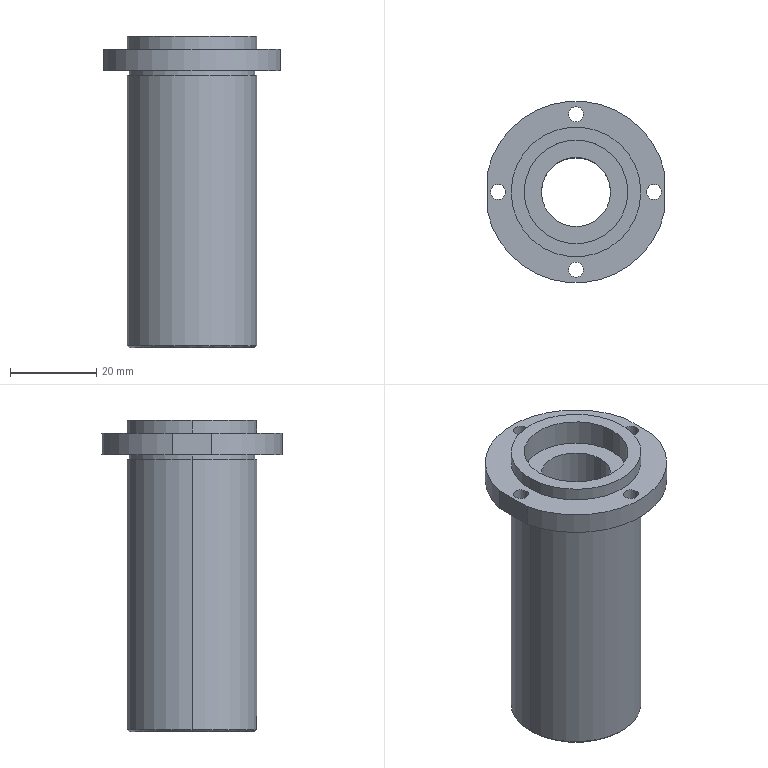Part | STEP file | 06-01-04 rotary shaft sleeve | 1 solid | 33 faces | box 41 x 42 x 72 mm | volume 36513 mm3 | cylinder 22 | plane 9 | cone 2 | commonest cylinder face diameters 3.5 x8 24 x4 30 x4 16 x2 29 x2 42 x2
STEP:
#1=CARTESIAN_POINT('',(-14.5,0.,0.));
#2=VERTEX_POINT('',#1);
#3=CARTESIAN_POINT('',(14.5,0.,0.));
#4=VERTEX_POINT('',#3);
#5=CARTESIAN_POINT('',(0.,0.,0.));
#6=DIRECTION('',(0.,0.,-1.));
#7=DIRECTION('',(1.,0.,0.));
#8=AXIS2_PLACEMENT_3D('',#5,#6,#7);
#9=CIRCLE('',#8,14.5);
#10=EDGE_CURVE('',#2,#4,#9,.T.);
#11=ORIENTED_EDGE('',*,*,#10,.F.);
#12=CARTESIAN_POINT('',(-15.,0.,0.5));
#13=VERTEX_POINT('',#12);
#14=CARTESIAN_POINT('',(-15.,0.,0.5));
#15=DIRECTION('',(-0.7071,0.,0.7071));
#16=VECTOR('',#15,1000.);
#17=LINE('',#14,#16);
#18=EDGE_CURVE('',#2,#13,#17,.T.);
#19=ORIENTED_EDGE('',*,*,#18,.T.);
#20=CARTESIAN_POINT('',(15.,0.,0.5));
#21=VERTEX_POINT('',#20);
#22=CARTESIAN_POINT('',(0.,0.,0.5));
#23=DIRECTION('',(0.,0.,1.));
#24=DIRECTION('',(1.,0.,0.));
#25=AXIS2_PLACEMENT_3D('',#22,#23,#24);
#26=CIRCLE('',#25,15.);
#27=EDGE_CURVE('',#21,#13,#26,.T.);
#28=ORIENTED_EDGE('',*,*,#27,.F.);
#29=CARTESIAN_POINT('',(15.,0.,0.5));
#30=DIRECTION('',(0.7071,0.,0.7071));
#31=VECTOR('',#30,1000.);
#32=LINE('',#29,#31);
#33=EDGE_CURVE('',#4,#21,#32,.T.);
#34=ORIENTED_EDGE('',*,*,#33,.F.);
#35=EDGE_LOOP('',(#11,#19,#28,#34));
#36=FACE_OUTER_BOUND('',#35,.T.);
#37=CARTESIAN_POINT('',(0.,0.,0.5));
#38=DIRECTION('',(0.,0.,1.));
#39=DIRECTION('',(1.,0.,0.));
#40=AXIS2_PLACEMENT_3D('',#37,#38,#39);
#41=CONICAL_SURFACE('',#40,15.,0.7854);
#42=ADVANCED_FACE('',(#36),#41,.T.);
#43=CARTESIAN_POINT('',(-14.5,0.,63.));
#44=VERTEX_POINT('',#43);
#45=CARTESIAN_POINT('',(14.5,0.,63.));
#46=VERTEX_POINT('',#45);
#47=CARTESIAN_POINT('',(0.,0.,63.));
#48=DIRECTION('',(0.,0.,-1.));
#49=DIRECTION('',(-1.,0.,0.));
#50=AXIS2_PLACEMENT_3D('',#47,#48,#49);
#51=CIRCLE('',#50,14.5);
#52=EDGE_CURVE('',#44,#46,#51,.T.);
#53=ORIENTED_EDGE('',*,*,#52,.F.);
#54=CARTESIAN_POINT('',(-14.5,0.,64.));
#55=VERTEX_POINT('',#54);
#56=CARTESIAN_POINT('',(-14.5,0.,63.));
#57=DIRECTION('',(0.,0.,1.));
#58=VECTOR('',#57,1000.);
#59=LINE('',#56,#58);
#60=EDGE_CURVE('',#44,#55,#59,.T.);
#61=ORIENTED_EDGE('',*,*,#60,.T.);
#62=CARTESIAN_POINT('',(14.5,0.,64.));
#63=VERTEX_POINT('',#62);
#64=CARTESIAN_POINT('',(0.,0.,64.));
#65=DIRECTION('',(0.,0.,-1.));
#66=DIRECTION('',(-1.,0.,0.));
#67=AXIS2_PLACEMENT_3D('',#64,#65,#66);
#68=CIRCLE('',#67,14.5);
#69=EDGE_CURVE('',#55,#63,#68,.T.);
#70=ORIENTED_EDGE('',*,*,#69,.T.);
#71=CARTESIAN_POINT('',(14.5,0.,63.));
#72=DIRECTION('',(0.,0.,1.));
#73=VECTOR('',#72,1000.);
#74=LINE('',#71,#73);
#75=EDGE_CURVE('',#46,#63,#74,.T.);
#76=ORIENTED_EDGE('',*,*,#75,.F.);
#77=EDGE_LOOP('',(#53,#61,#70,#76));
#78=FACE_OUTER_BOUND('',#77,.T.);
#79=CARTESIAN_POINT('',(0.,0.,63.));
#80=DIRECTION('',(0.,0.,1.));
#81=DIRECTION('',(1.,0.,0.));
#82=AXIS2_PLACEMENT_3D('',#79,#80,#81);
#83=CYLINDRICAL_SURFACE('',#82,14.5);
#84=ADVANCED_FACE('',(#78),#83,.T.);
#85=CARTESIAN_POINT('',(-19.75,0.,64.));
#86=VERTEX_POINT('',#85);
#87=CARTESIAN_POINT('',(-16.25,0.,64.));
#88=VERTEX_POINT('',#87);
#89=CARTESIAN_POINT('',(-18.,0.,64.));
#90=DIRECTION('',(0.,0.,1.));
#91=DIRECTION('',(1.,0.,0.));
#92=AXIS2_PLACEMENT_3D('',#89,#90,#91);
#93=CIRCLE('',#92,1.75);
#94=EDGE_CURVE('',#86,#88,#93,.T.);
#95=ORIENTED_EDGE('',*,*,#94,.F.);
#96=CARTESIAN_POINT('',(-19.75,0.,69.));
#97=VERTEX_POINT('',#96);
#98=CARTESIAN_POINT('',(-19.75,0.,64.));
#99=DIRECTION('',(0.,0.,1.));
#100=VECTOR('',#99,1000.);
#101=LINE('',#98,#100);
#102=EDGE_CURVE('',#86,#97,#101,.T.);
#103=ORIENTED_EDGE('',*,*,#102,.T.);
#104=CARTESIAN_POINT('',(-16.25,0.,69.));
#105=VERTEX_POINT('',#104);
#106=CARTESIAN_POINT('',(-18.,0.,69.));
#107=DIRECTION('',(0.,0.,1.));
#108=DIRECTION('',(1.,0.,0.));
#109=AXIS2_PLACEMENT_3D('',#106,#107,#108);
#110=CIRCLE('',#109,1.75);
#111=EDGE_CURVE('',#97,#105,#110,.T.);
#112=ORIENTED_EDGE('',*,*,#111,.T.);
#113=CARTESIAN_POINT('',(-16.25,0.,64.));
#114=DIRECTION('',(0.,0.,1.));
#115=VECTOR('',#114,1000.);
#116=LINE('',#113,#115);
#117=EDGE_CURVE('',#88,#105,#116,.T.);
#118=ORIENTED_EDGE('',*,*,#117,.F.);
#119=EDGE_LOOP('',(#95,#103,#112,#118));
#120=FACE_OUTER_BOUND('',#119,.T.);
#121=CARTESIAN_POINT('',(-18.,0.,64.));
#122=DIRECTION('',(0.,0.,1.));
#123=DIRECTION('',(1.,0.,0.));
#124=AXIS2_PLACEMENT_3D('',#121,#122,#123);
#125=CYLINDRICAL_SURFACE('',#124,1.75);
#126=ADVANCED_FACE('',(#120),#125,.F.);
#127=CARTESIAN_POINT('',(16.25,0.,64.));
#128=VERTEX_POINT('',#127);
#129=CARTESIAN_POINT('',(19.75,0.,64.));
#130=VERTEX_POINT('',#129);
#131=CARTESIAN_POINT('',(18.,0.,64.));
#132=DIRECTION('',(0.,0.,1.));
#133=DIRECTION('',(1.,0.,0.));
#134=AXIS2_PLACEMENT_3D('',#131,#132,#133);
#135=CIRCLE('',#134,1.75);
#136=EDGE_CURVE('',#128,#130,#135,.T.);
#137=ORIENTED_EDGE('',*,*,#136,.F.);
#138=CARTESIAN_POINT('',(16.25,0.,69.));
#139=VERTEX_POINT('',#138);
#140=CARTESIAN_POINT('',(16.25,0.,64.));
#141=DIRECTION('',(0.,0.,1.));
#142=VECTOR('',#141,1000.);
#143=LINE('',#140,#142);
#144=EDGE_CURVE('',#128,#139,#143,.T.);
#145=ORIENTED_EDGE('',*,*,#144,.T.);
#146=CARTESIAN_POINT('',(19.75,0.,69.));
#147=VERTEX_POINT('',#146);
#148=CARTESIAN_POINT('',(18.,0.,69.));
#149=DIRECTION('',(0.,0.,1.));
#150=DIRECTION('',(1.,0.,0.));
#151=AXIS2_PLACEMENT_3D('',#148,#149,#150);
#152=CIRCLE('',#151,1.75);
#153=EDGE_CURVE('',#139,#147,#152,.T.);
#154=ORIENTED_EDGE('',*,*,#153,.T.);
#155=CARTESIAN_POINT('',(19.75,0.,64.));
#156=DIRECTION('',(0.,0.,1.));
#157=VECTOR('',#156,1000.);
#158=LINE('',#155,#157);
#159=EDGE_CURVE('',#130,#147,#158,.T.);
#160=ORIENTED_EDGE('',*,*,#159,.F.);
#161=EDGE_LOOP('',(#137,#145,#154,#160));
#162=FACE_OUTER_BOUND('',#161,.T.);
#163=CARTESIAN_POINT('',(18.,0.,64.));
#164=DIRECTION('',(0.,0.,1.));
#165=DIRECTION('',(1.,0.,0.));
#166=AXIS2_PLACEMENT_3D('',#163,#164,#165);
#167=CYLINDRICAL_SURFACE('',#166,1.75);
#168=ADVANCED_FACE('',(#162),#167,.F.);
#169=CARTESIAN_POINT('',(-1.75,-18.,64.));
#170=VERTEX_POINT('',#169);
#171=CARTESIAN_POINT('',(1.75,-18.,64.));
#172=VERTEX_POINT('',#171);
#173=CARTESIAN_POINT('',(0.,-18.,64.));
#174=DIRECTION('',(0.,0.,1.));
#175=DIRECTION('',(1.,0.,0.));
#176=AXIS2_PLACEMENT_3D('',#173,#174,#175);
#177=CIRCLE('',#176,1.75);
#178=EDGE_CURVE('',#170,#172,#177,.T.);
#179=ORIENTED_EDGE('',*,*,#178,.F.);
#180=CARTESIAN_POINT('',(-1.75,-18.,69.));
#181=VERTEX_POINT('',#180);
#182=CARTESIAN_POINT('',(-1.75,-18.,64.));
#183=DIRECTION('',(0.,0.,1.));
#184=VECTOR('',#183,1000.);
#185=LINE('',#182,#184);
#186=EDGE_CURVE('',#170,#181,#185,.T.);
#187=ORIENTED_EDGE('',*,*,#186,.T.);
#188=CARTESIAN_POINT('',(1.75,-18.,69.));
#189=VERTEX_POINT('',#188);
#190=CARTESIAN_POINT('',(0.,-18.,69.));
#191=DIRECTION('',(0.,0.,1.));
#192=DIRECTION('',(1.,0.,0.));
#193=AXIS2_PLACEMENT_3D('',#190,#191,#192);
#194=CIRCLE('',#193,1.75);
#195=EDGE_CURVE('',#181,#189,#194,.T.);
#196=ORIENTED_EDGE('',*,*,#195,.T.);
#197=CARTESIAN_POINT('',(1.75,-18.,64.));
#198=DIRECTION('',(0.,0.,1.));
#199=VECTOR('',#198,1000.);
#200=LINE('',#197,#199);
#201=EDGE_CURVE('',#172,#189,#200,.T.);
#202=ORIENTED_EDGE('',*,*,#201,.F.);
#203=EDGE_LOOP('',(#179,#187,#196,#202));
#204=FACE_OUTER_BOUND('',#203,.T.);
#205=CARTESIAN_POINT('',(0.,-18.,64.));
#206=DIRECTION('',(0.,0.,1.));
#207=DIRECTION('',(1.,0.,0.));
#208=AXIS2_PLACEMENT_3D('',#205,#206,#207);
#209=CYLINDRICAL_SURFACE('',#208,1.75);
#210=ADVANCED_FACE('',(#204),#209,.F.);
#211=CARTESIAN_POINT('',(-1.75,18.,64.));
#212=VERTEX_POINT('',#211);
#213=CARTESIAN_POINT('',(1.75,18.,64.));
#214=VERTEX_POINT('',#213);
#215=CARTESIAN_POINT('',(0.,18.,64.));
#216=DIRECTION('',(0.,0.,1.));
#217=DIRECTION('',(1.,0.,0.));
#218=AXIS2_PLACEMENT_3D('',#215,#216,#217);
#219=CIRCLE('',#218,1.75);
#220=EDGE_CURVE('',#212,#214,#219,.T.);
#221=ORIENTED_EDGE('',*,*,#220,.F.);
#222=CARTESIAN_POINT('',(-1.75,18.,69.));
#223=VERTEX_POINT('',#222);
#224=CARTESIAN_POINT('',(-1.75,18.,64.));
#225=DIRECTION('',(0.,0.,1.));
#226=VECTOR('',#225,1000.);
#227=LINE('',#224,#226);
#228=EDGE_CURVE('',#212,#223,#227,.T.);
#229=ORIENTED_EDGE('',*,*,#228,.T.);
#230=CARTESIAN_POINT('',(1.75,18.,69.));
#231=VERTEX_POINT('',#230);
#232=CARTESIAN_POINT('',(0.,18.,69.));
#233=DIRECTION('',(0.,0.,1.));
#234=DIRECTION('',(1.,0.,0.));
#235=AXIS2_PLACEMENT_3D('',#232,#233,#234);
#236=CIRCLE('',#235,1.75);
#237=EDGE_CURVE('',#223,#231,#236,.T.);
#238=ORIENTED_EDGE('',*,*,#237,.T.);
#239=CARTESIAN_POINT('',(1.75,18.,64.));
#240=DIRECTION('',(0.,0.,1.));
#241=VECTOR('',#240,1000.);
#242=LINE('',#239,#241);
#243=EDGE_CURVE('',#214,#231,#242,.T.);
#244=ORIENTED_EDGE('',*,*,#243,.F.);
#245=EDGE_LOOP('',(#221,#229,#238,#244));
#246=FACE_OUTER_BOUND('',#245,.T.);
#247=CARTESIAN_POINT('',(0.,18.,64.));
#248=DIRECTION('',(0.,0.,1.));
#249=DIRECTION('',(1.,0.,0.));
#250=AXIS2_PLACEMENT_3D('',#247,#248,#249);
#251=CYLINDRICAL_SURFACE('',#250,1.75);
#252=ADVANCED_FACE('',(#246),#251,.F.);
#253=CARTESIAN_POINT('',(8.,0.,6.));
#254=VERTEX_POINT('',#253);
#255=CARTESIAN_POINT('',(-8.,0.,6.));
#256=VERTEX_POINT('',#255);
#257=CARTESIAN_POINT('',(0.,0.,6.));
#258=DIRECTION('',(0.,0.,-1.));
#259=DIRECTION('',(-1.,0.,0.));
#260=AXIS2_PLACEMENT_3D('',#257,#258,#259);
#261=CIRCLE('',#260,8.);
#262=EDGE_CURVE('',#254,#256,#261,.T.);
#263=ORIENTED_EDGE('',*,*,#262,.T.);
#264=CARTESIAN_POINT('',(-8.,0.,66.));
#265=VERTEX_POINT('',#264);
#266=CARTESIAN_POINT('',(-8.,0.,0.));
#267=DIRECTION('',(0.,0.,1.));
#268=VECTOR('',#267,1000.);
#269=LINE('',#266,#268);
#270=EDGE_CURVE('',#256,#265,#269,.T.);
#271=ORIENTED_EDGE('',*,*,#270,.T.);
#272=CARTESIAN_POINT('',(8.,0.,66.));
#273=VERTEX_POINT('',#272);
#274=CARTESIAN_POINT('',(0.,0.,66.));
#275=DIRECTION('',(0.,0.,1.));
#276=DIRECTION('',(1.,0.,0.));
#277=AXIS2_PLACEMENT_3D('',#274,#275,#276);
#278=CIRCLE('',#277,8.);
#279=EDGE_CURVE('',#265,#273,#278,.T.);
#280=ORIENTED_EDGE('',*,*,#279,.T.);
#281=CARTESIAN_POINT('',(8.,0.,0.));
#282=DIRECTION('',(0.,0.,1.));
#283=VECTOR('',#282,1000.);
#284=LINE('',#281,#283);
#285=EDGE_CURVE('',#254,#273,#284,.T.);
#286=ORIENTED_EDGE('',*,*,#285,.F.);
#287=EDGE_LOOP('',(#263,#271,#280,#286));
#288=FACE_OUTER_BOUND('',#287,.T.);
#289=CARTESIAN_POINT('',(0.,0.,0.));
#290=DIRECTION('',(0.,0.,1.));
#291=DIRECTION('',(1.,0.,0.));
#292=AXIS2_PLACEMENT_3D('',#289,#290,#291);
#293=CYLINDRICAL_SURFACE('',#292,8.);
#294=ADVANCED_FACE('',(#288),#293,.F.);
#295=CARTESIAN_POINT('',(-12.,0.,66.));
#296=VERTEX_POINT('',#295);
#297=CARTESIAN_POINT('',(12.,0.,66.));
#298=VERTEX_POINT('',#297);
#299=CARTESIAN_POINT('',(0.,0.,66.));
#300=DIRECTION('',(0.,0.,1.));
#301=DIRECTION('',(1.,0.,0.));
#302=AXIS2_PLACEMENT_3D('',#299,#300,#301);
#303=CIRCLE('',#302,12.);
#304=EDGE_CURVE('',#296,#298,#303,.T.);
#305=ORIENTED_EDGE('',*,*,#304,.F.);
#306=CARTESIAN_POINT('',(-12.,0.,72.));
#307=VERTEX_POINT('',#306);
#308=CARTESIAN_POINT('',(-12.,0.,66.));
#309=DIRECTION('',(0.,0.,1.));
#310=VECTOR('',#309,1000.);
#311=LINE('',#308,#310);
#312=EDGE_CURVE('',#296,#307,#311,.T.);
#313=ORIENTED_EDGE('',*,*,#312,.T.);
#314=CARTESIAN_POINT('',(12.,0.,72.));
#315=VERTEX_POINT('',#314);
#316=CARTESIAN_POINT('',(0.,0.,72.));
#317=DIRECTION('',(0.,0.,1.));
#318=DIRECTION('',(1.,0.,0.));
#319=AXIS2_PLACEMENT_3D('',#316,#317,#318);
#320=CIRCLE('',#319,12.);
#321=EDGE_CURVE('',#307,#315,#320,.T.);
#322=ORIENTED_EDGE('',*,*,#321,.T.);
#323=CARTESIAN_POINT('',(12.,0.,66.));
#324=DIRECTION('',(0.,0.,1.));
#325=VECTOR('',#324,1000.);
#326=LINE('',#323,#325);
#327=EDGE_CURVE('',#298,#315,#326,.T.);
#328=ORIENTED_EDGE('',*,*,#327,.F.);
#329=EDGE_LOOP('',(#305,#313,#322,#328));
#330=FACE_OUTER_BOUND('',#329,.T.);
#331=CARTESIAN_POINT('',(0.,0.,66.));
#332=DIRECTION('',(0.,0.,1.));
#333=DIRECTION('',(1.,0.,0.));
#334=AXIS2_PLACEMENT_3D('',#331,#332,#333);
#335=CYLINDRICAL_SURFACE('',#334,12.);
#336=ADVANCED_FACE('',(#330),#335,.F.);
#337=CARTESIAN_POINT('',(12.,0.,6.));
#338=VERTEX_POINT('',#337);
#339=CARTESIAN_POINT('',(-12.,0.,6.));
#340=VERTEX_POINT('',#339);
#341=CARTESIAN_POINT('',(0.,0.,6.));
#342=DIRECTION('',(0.,0.,-1.));
#343=DIRECTION('',(-1.,0.,0.));
#344=AXIS2_PLACEMENT_3D('',#341,#342,#343);
#345=CIRCLE('',#344,12.);
#346=EDGE_CURVE('',#338,#340,#345,.T.);
#347=ORIENTED_EDGE('',*,*,#346,.F.);
#348=CARTESIAN_POINT('',(12.,0.,0.));
#349=VERTEX_POINT('',#348);
#350=CARTESIAN_POINT('',(12.,0.,6.));
#351=DIRECTION('',(0.,0.,-1.));
#352=VECTOR('',#351,1000.);
#353=LINE('',#350,#352);
#354=EDGE_CURVE('',#338,#349,#353,.T.);
#355=ORIENTED_EDGE('',*,*,#354,.T.);
#356=CARTESIAN_POINT('',(-12.,0.,0.));
#357=VERTEX_POINT('',#356);
#358=CARTESIAN_POINT('',(0.,0.,0.));
#359=DIRECTION('',(0.,0.,-1.));
#360=DIRECTION('',(-1.,0.,0.));
#361=AXIS2_PLACEMENT_3D('',#358,#359,#360);
#362=CIRCLE('',#361,12.);
#363=EDGE_CURVE('',#349,#357,#362,.T.);
#364=ORIENTED_EDGE('',*,*,#363,.T.);
#365=CARTESIAN_POINT('',(-12.,0.,6.));
#366=DIRECTION('',(0.,0.,-1.));
#367=VECTOR('',#366,1000.);
#368=LINE('',#365,#367);
#369=EDGE_CURVE('',#340,#357,#368,.T.);
#370=ORIENTED_EDGE('',*,*,#369,.F.);
#371=EDGE_LOOP('',(#347,#355,#364,#370));
#372=FACE_OUTER_BOUND('',#371,.T.);
#373=CARTESIAN_POINT('',(0.,0.,6.));
#374=DIRECTION('',(0.,0.,-1.));
#375=DIRECTION('',(-1.,0.,0.));
#376=AXIS2_PLACEMENT_3D('',#373,#374,#375);
#377=CYLINDRICAL_SURFACE('',#376,12.);
#378=ADVANCED_FACE('',(#372),#377,.F.);
#379=CARTESIAN_POINT('',(15.,0.,72.));
#380=VERTEX_POINT('',#379);
#381=CARTESIAN_POINT('',(-15.,0.,72.));
#382=VERTEX_POINT('',#381);
#383=CARTESIAN_POINT('',(0.,0.,72.));
#384=DIRECTION('',(0.,0.,1.));
#385=DIRECTION('',(1.,0.,0.));
#386=AXIS2_PLACEMENT_3D('',#383,#384,#385);
#387=CIRCLE('',#386,15.);
#388=EDGE_CURVE('',#380,#382,#387,.T.);
#389=ORIENTED_EDGE('',*,*,#388,.F.);
#390=CARTESIAN_POINT('',(15.,0.,69.));
#391=VERTEX_POINT('',#390);
#392=CARTESIAN_POINT('',(15.,0.,72.));
#393=DIRECTION('',(0.,0.,-1.));
#394=VECTOR('',#393,1000.);
#395=LINE('',#392,#394);
#396=EDGE_CURVE('',#380,#391,#395,.T.);
#397=ORIENTED_EDGE('',*,*,#396,.T.);
#398=CARTESIAN_POINT('',(-15.,0.,69.));
#399=VERTEX_POINT('',#398);
#400=CARTESIAN_POINT('',(0.,0.,69.));
#401=DIRECTION('',(0.,0.,1.));
#402=DIRECTION('',(1.,0.,0.));
#403=AXIS2_PLACEMENT_3D('',#400,#401,#402);
#404=CIRCLE('',#403,15.);
#405=EDGE_CURVE('',#391,#399,#404,.T.);
#406=ORIENTED_EDGE('',*,*,#405,.T.);
#407=CARTESIAN_POINT('',(-15.,0.,72.));
#408=DIRECTION('',(0.,0.,-1.));
#409=VECTOR('',#408,1000.);
#410=LINE('',#407,#409);
#411=EDGE_CURVE('',#382,#399,#410,.T.);
#412=ORIENTED_EDGE('',*,*,#411,.F.);
#413=EDGE_LOOP('',(#389,#397,#406,#412));
#414=FACE_OUTER_BOUND('',#413,.T.);
#415=CARTESIAN_POINT('',(0.,0.,72.));
#416=DIRECTION('',(0.,0.,-1.));
#417=DIRECTION('',(-1.,0.,0.));
#418=AXIS2_PLACEMENT_3D('',#415,#416,#417);
#419=CYLINDRICAL_SURFACE('',#418,15.);
#420=ADVANCED_FACE('',(#414),#419,.T.);
#421=CARTESIAN_POINT('',(-15.,0.,63.));
#422=VERTEX_POINT('',#421);
#423=CARTESIAN_POINT('',(15.,0.,63.));
#424=VERTEX_POINT('',#423);
#425=CARTESIAN_POINT('',(0.,0.,63.));
#426=DIRECTION('',(0.,0.,-1.));
#427=DIRECTION('',(-1.,0.,0.));
#428=AXIS2_PLACEMENT_3D('',#425,#426,#427);
#429=CIRCLE('',#428,15.);
#430=EDGE_CURVE('',#422,#424,#429,.T.);
#431=ORIENTED_EDGE('',*,*,#430,.T.);
#432=CARTESIAN_POINT('',(15.,0.,72.));
#433=DIRECTION('',(0.,0.,-1.));
#434=VECTOR('',#433,1000.);
#435=LINE('',#432,#434);
#436=EDGE_CURVE('',#424,#21,#435,.T.);
#437=ORIENTED_EDGE('',*,*,#436,.T.);
#438=ORIENTED_EDGE('',*,*,#27,.T.);
#439=CARTESIAN_POINT('',(-15.,0.,72.));
#440=DIRECTION('',(0.,0.,-1.));
#441=VECTOR('',#440,1000.);
#442=LINE('',#439,#441);
#443=EDGE_CURVE('',#422,#13,#442,.T.);
#444=ORIENTED_EDGE('',*,*,#443,.F.);
#445=EDGE_LOOP('',(#431,#437,#438,#444));
#446=FACE_OUTER_BOUND('',#445,.T.);
#447=CARTESIAN_POINT('',(0.,0.,72.));
#448=DIRECTION('',(0.,0.,-1.));
#449=DIRECTION('',(-1.,0.,0.));
#450=AXIS2_PLACEMENT_3D('',#447,#448,#449);
#451=CYLINDRICAL_SURFACE('',#450,15.);
#452=ADVANCED_FACE('',(#446),#451,.T.);
#453=CARTESIAN_POINT('',(-20.5,4.555,69.));
#454=VERTEX_POINT('',#453);
#455=CARTESIAN_POINT('',(-20.5,4.555,64.));
#456=VERTEX_POINT('',#455);
#457=CARTESIAN_POINT('',(-20.5,4.555,64.));
#458=DIRECTION('',(0.,0.,-1.));
#459=VECTOR('',#458,1000.);
#460=LINE('',#457,#459);
#461=EDGE_CURVE('',#454,#456,#460,.T.);
#462=ORIENTED_EDGE('',*,*,#461,.F.);
#463=CARTESIAN_POINT('',(20.5,4.555,69.));
#464=VERTEX_POINT('',#463);
#465=CARTESIAN_POINT('',(0.,0.,69.));
#466=DIRECTION('',(0.,0.,1.));
#467=DIRECTION('',(1.,0.,0.));
#468=AXIS2_PLACEMENT_3D('',#465,#466,#467);
#469=CIRCLE('',#468,21.);
#470=EDGE_CURVE('',#464,#454,#469,.T.);
#471=ORIENTED_EDGE('',*,*,#470,.F.);
#472=CARTESIAN_POINT('',(20.5,4.555,64.));
#473=VERTEX_POINT('',#472);
#474=CARTESIAN_POINT('',(20.5,4.555,64.));
#475=DIRECTION('',(0.,0.,1.));
#476=VECTOR('',#475,1000.);
#477=LINE('',#474,#476);
#478=EDGE_CURVE('',#473,#464,#477,.T.);
#479=ORIENTED_EDGE('',*,*,#478,.F.);
#480=CARTESIAN_POINT('',(0.,0.,64.));
#481=DIRECTION('',(0.,0.,1.));
#482=DIRECTION('',(1.,0.,0.));
#483=AXIS2_PLACEMENT_3D('',#480,#481,#482);
#484=CIRCLE('',#483,21.);
#485=EDGE_CURVE('',#473,#456,#484,.T.);
#486=ORIENTED_EDGE('',*,*,#485,.T.);
#487=EDGE_LOOP('',(#462,#471,#479,#486));
#488=FACE_OUTER_BOUND('',#487,.T.);
#489=CARTESIAN_POINT('',(0.,0.,64.));
#490=DIRECTION('',(0.,0.,1.));
#491=DIRECTION('',(1.,0.,0.));
#492=AXIS2_PLACEMENT_3D('',#489,#490,#491);
#493=CYLINDRICAL_SURFACE('',#492,21.);
#494=ADVANCED_FACE('',(#488),#493,.T.);
#495=ORIENTED_EDGE('',*,*,#436,.F.);
#496=CARTESIAN_POINT('',(0.,0.,63.));
#497=DIRECTION('',(0.,0.,-1.));
#498=DIRECTION('',(-1.,0.,0.));
#499=AXIS2_PLACEMENT_3D('',#496,#497,#498);
#500=CIRCLE('',#499,15.);
#501=EDGE_CURVE('',#424,#422,#500,.T.);
#502=ORIENTED_EDGE('',*,*,#501,.T.);
#503=ORIENTED_EDGE('',*,*,#443,.T.);
#504=CARTESIAN_POINT('',(0.,0.,0.5));
#505=DIRECTION('',(0.,0.,1.));
#506=DIRECTION('',(1.,0.,0.));
#507=AXIS2_PLACEMENT_3D('',#504,#505,#506);
#508=CIRCLE('',#507,15.);
#509=EDGE_CURVE('',#13,#21,#508,.T.);
#510=ORIENTED_EDGE('',*,*,#509,.T.);
#511=EDGE_LOOP('',(#495,#502,#503,#510));
#512=FACE_OUTER_BOUND('',#511,.T.);
#513=CARTESIAN_POINT('',(0.,0.,72.));
#514=DIRECTION('',(0.,0.,-1.));
#515=DIRECTION('',(-1.,0.,0.));
#516=AXIS2_PLACEMENT_3D('',#513,#514,#515);
#517=CYLINDRICAL_SURFACE('',#516,15.);
#518=ADVANCED_FACE('',(#512),#517,.T.);
#519=ORIENTED_EDGE('',*,*,#396,.F.);
#520=CARTESIAN_POINT('',(0.,0.,72.));
#521=DIRECTION('',(0.,0.,1.));
#522=DIRECTION('',(1.,0.,0.));
#523=AXIS2_PLACEMENT_3D('',#520,#521,#522);
#524=CIRCLE('',#523,15.);
#525=EDGE_CURVE('',#382,#380,#524,.T.);
#526=ORIENTED_EDGE('',*,*,#525,.F.);
#527=ORIENTED_EDGE('',*,*,#411,.T.);
#528=CARTESIAN_POINT('',(0.,0.,69.));
#529=DIRECTION('',(0.,0.,1.));
#530=DIRECTION('',(1.,0.,0.));
#531=AXIS2_PLACEMENT_3D('',#528,#529,#530);
#532=CIRCLE('',#531,15.);
#533=EDGE_CURVE('',#399,#391,#532,.T.);
#534=ORIENTED_EDGE('',*,*,#533,.T.);
#535=EDGE_LOOP('',(#519,#526,#527,#534));
#536=FACE_OUTER_BOUND('',#535,.T.);
#537=CARTESIAN_POINT('',(0.,0.,72.));
#538=DIRECTION('',(0.,0.,-1.));
#539=DIRECTION('',(-1.,0.,0.));
#540=AXIS2_PLACEMENT_3D('',#537,#538,#539);
#541=CYLINDRICAL_SURFACE('',#540,15.);
#542=ADVANCED_FACE('',(#536),#541,.T.);
#543=CARTESIAN_POINT('',(0.,0.,72.));
#544=DIRECTION('',(0.,0.,1.));
#545=DIRECTION('',(1.,0.,0.));
#546=AXIS2_PLACEMENT_3D('',#543,#544,#545);
#547=CIRCLE('',#546,12.);
#548=EDGE_CURVE('',#315,#307,#547,.T.);
#549=ORIENTED_EDGE('',*,*,#548,.F.);
#550=ORIENTED_EDGE('',*,*,#321,.F.);
#551=EDGE_LOOP('',(#549,#550));
#552=FACE_BOUND('',#551,.T.);
#553=ORIENTED_EDGE('',*,*,#525,.T.);
#554=ORIENTED_EDGE('',*,*,#388,.T.);
#555=EDGE_LOOP('',(#553,#554));
#556=FACE_OUTER_BOUND('',#555,.T.);
#557=CARTESIAN_POINT('',(0.,0.,72.));
#558=DIRECTION('',(0.,0.,1.));
#559=DIRECTION('',(1.,0.,0.));
#560=AXIS2_PLACEMENT_3D('',#557,#558,#559);
#561=PLANE('',#560);
#562=ADVANCED_FACE('',(#552,#556),#561,.T.);
#563=CARTESIAN_POINT('',(0.,0.,0.));
#564=DIRECTION('',(0.,0.,-1.));
#565=DIRECTION('',(1.,0.,0.));
#566=AXIS2_PLACEMENT_3D('',#563,#564,#565);
#567=CIRCLE('',#566,14.5);
#568=EDGE_CURVE('',#4,#2,#567,.T.);
#569=ORIENTED_EDGE('',*,*,#568,.T.);
#570=ORIENTED_EDGE('',*,*,#10,.T.);
#571=EDGE_LOOP('',(#569,#570));
#572=FACE_OUTER_BOUND('',#571,.T.);
#573=CARTESIAN_POINT('',(0.,0.,0.));
#574=DIRECTION('',(0.,0.,-1.));
#575=DIRECTION('',(-1.,0.,0.));
#576=AXIS2_PLACEMENT_3D('',#573,#574,#575);
#577=CIRCLE('',#576,12.);
#578=EDGE_CURVE('',#357,#349,#577,.T.);
#579=ORIENTED_EDGE('',*,*,#578,.F.);
#580=ORIENTED_EDGE('',*,*,#363,.F.);
#581=EDGE_LOOP('',(#579,#580));
#582=FACE_BOUND('',#581,.T.);
#583=CARTESIAN_POINT('',(0.,0.,0.));
#584=DIRECTION('',(0.,0.,1.));
#585=DIRECTION('',(1.,0.,0.));
#586=AXIS2_PLACEMENT_3D('',#583,#584,#585);
#587=PLANE('',#586);
#588=ADVANCED_FACE('',(#572,#582),#587,.F.);
#589=ORIENTED_EDGE('',*,*,#354,.F.);
#590=CARTESIAN_POINT('',(0.,0.,6.));
#591=DIRECTION('',(0.,0.,-1.));
#592=DIRECTION('',(-1.,0.,0.));
#593=AXIS2_PLACEMENT_3D('',#590,#591,#592);
#594=CIRCLE('',#593,12.);
#595=EDGE_CURVE('',#340,#338,#594,.T.);
#596=ORIENTED_EDGE('',*,*,#595,.F.);
#597=ORIENTED_EDGE('',*,*,#369,.T.);
#598=ORIENTED_EDGE('',*,*,#578,.T.);
#599=EDGE_LOOP('',(#589,#596,#597,#598));
#600=FACE_OUTER_BOUND('',#599,.T.);
#601=CARTESIAN_POINT('',(0.,0.,6.));
#602=DIRECTION('',(0.,0.,-1.));
#603=DIRECTION('',(-1.,0.,0.));
#604=AXIS2_PLACEMENT_3D('',#601,#602,#603);
#605=CYLINDRICAL_SURFACE('',#604,12.);
#606=ADVANCED_FACE('',(#600),#605,.F.);
#607=ORIENTED_EDGE('',*,*,#262,.F.);
#608=CARTESIAN_POINT('',(0.,0.,6.));
#609=DIRECTION('',(0.,0.,-1.));
#610=DIRECTION('',(-1.,0.,0.));
#611=AXIS2_PLACEMENT_3D('',#608,#609,#610);
#612=CIRCLE('',#611,8.);
#613=EDGE_CURVE('',#256,#254,#612,.T.);
#614=ORIENTED_EDGE('',*,*,#613,.F.);
#615=EDGE_LOOP('',(#607,#614));
#616=FACE_BOUND('',#615,.T.);
#617=ORIENTED_EDGE('',*,*,#595,.T.);
#618=ORIENTED_EDGE('',*,*,#346,.T.);
#619=EDGE_LOOP('',(#617,#618));
#620=FACE_OUTER_BOUND('',#619,.T.);
#621=CARTESIAN_POINT('',(0.,0.,6.));
#622=DIRECTION('',(0.,0.,-1.));
#623=DIRECTION('',(-1.,0.,0.));
#624=AXIS2_PLACEMENT_3D('',#621,#622,#623);
#625=PLANE('',#624);
#626=ADVANCED_FACE('',(#616,#620),#625,.T.);
#627=ORIENTED_EDGE('',*,*,#312,.F.);
#628=CARTESIAN_POINT('',(0.,0.,66.));
#629=DIRECTION('',(0.,0.,1.));
#630=DIRECTION('',(1.,0.,0.));
#631=AXIS2_PLACEMENT_3D('',#628,#629,#630);
#632=CIRCLE('',#631,12.);
#633=EDGE_CURVE('',#298,#296,#632,.T.);
#634=ORIENTED_EDGE('',*,*,#633,.F.);
#635=ORIENTED_EDGE('',*,*,#327,.T.);
#636=ORIENTED_EDGE('',*,*,#548,.T.);
#637=EDGE_LOOP('',(#627,#634,#635,#636));
#638=FACE_OUTER_BOUND('',#637,.T.);
#639=CARTESIAN_POINT('',(0.,0.,66.));
#640=DIRECTION('',(0.,0.,1.));
#641=DIRECTION('',(1.,0.,0.));
#642=AXIS2_PLACEMENT_3D('',#639,#640,#641);
#643=CYLINDRICAL_SURFACE('',#642,12.);
#644=ADVANCED_FACE('',(#638),#643,.F.);
#645=CARTESIAN_POINT('',(0.,0.,66.));
#646=DIRECTION('',(0.,0.,1.));
#647=DIRECTION('',(1.,0.,0.));
#648=AXIS2_PLACEMENT_3D('',#645,#646,#647);
#649=CIRCLE('',#648,8.);
#650=EDGE_CURVE('',#273,#265,#649,.T.);
#651=ORIENTED_EDGE('',*,*,#650,.F.);
#652=ORIENTED_EDGE('',*,*,#279,.F.);
#653=EDGE_LOOP('',(#651,#652));
#654=FACE_BOUND('',#653,.T.);
#655=ORIENTED_EDGE('',*,*,#633,.T.);
#656=ORIENTED_EDGE('',*,*,#304,.T.);
#657=EDGE_LOOP('',(#655,#656));
#658=FACE_OUTER_BOUND('',#657,.T.);
#659=CARTESIAN_POINT('',(0.,0.,66.));
#660=DIRECTION('',(0.,0.,1.));
#661=DIRECTION('',(1.,0.,0.));
#662=AXIS2_PLACEMENT_3D('',#659,#660,#661);
#663=PLANE('',#662);
#664=ADVANCED_FACE('',(#654,#658),#663,.T.);
#665=ORIENTED_EDGE('',*,*,#270,.F.);
#666=ORIENTED_EDGE('',*,*,#613,.T.);
#667=ORIENTED_EDGE('',*,*,#285,.T.);
#668=ORIENTED_EDGE('',*,*,#650,.T.);
#669=EDGE_LOOP('',(#665,#666,#667,#668));
#670=FACE_OUTER_BOUND('',#669,.T.);
#671=CARTESIAN_POINT('',(0.,0.,0.));
#672=DIRECTION('',(0.,0.,1.));
#673=DIRECTION('',(1.,0.,0.));
#674=AXIS2_PLACEMENT_3D('',#671,#672,#673);
#675=CYLINDRICAL_SURFACE('',#674,8.);
#676=ADVANCED_FACE('',(#670),#675,.F.);
#677=CARTESIAN_POINT('',(-20.5,-4.555,64.));
#678=VERTEX_POINT('',#677);
#679=CARTESIAN_POINT('',(-20.5,-4.555,69.));
#680=VERTEX_POINT('',#679);
#681=CARTESIAN_POINT('',(-20.5,-4.555,64.));
#682=DIRECTION('',(0.,0.,1.));
#683=VECTOR('',#682,1000.);
#684=LINE('',#681,#683);
#685=EDGE_CURVE('',#678,#680,#684,.T.);
#686=ORIENTED_EDGE('',*,*,#685,.F.);
#687=CARTESIAN_POINT('',(20.5,-4.555,64.));
#688=VERTEX_POINT('',#687);
#689=CARTESIAN_POINT('',(0.,0.,64.));
#690=DIRECTION('',(0.,0.,1.));
#691=DIRECTION('',(1.,0.,0.));
#692=AXIS2_PLACEMENT_3D('',#689,#690,#691);
#693=CIRCLE('',#692,21.);
#694=EDGE_CURVE('',#678,#688,#693,.T.);
#695=ORIENTED_EDGE('',*,*,#694,.T.);
#696=CARTESIAN_POINT('',(20.5,-4.555,69.));
#697=VERTEX_POINT('',#696);
#698=CARTESIAN_POINT('',(20.5,-4.555,64.));
#699=DIRECTION('',(0.,0.,-1.));
#700=VECTOR('',#699,1000.);
#701=LINE('',#698,#700);
#702=EDGE_CURVE('',#697,#688,#701,.T.);
#703=ORIENTED_EDGE('',*,*,#702,.F.);
#704=CARTESIAN_POINT('',(0.,0.,69.));
#705=DIRECTION('',(0.,0.,1.));
#706=DIRECTION('',(1.,0.,0.));
#707=AXIS2_PLACEMENT_3D('',#704,#705,#706);
#708=CIRCLE('',#707,21.);
#709=EDGE_CURVE('',#680,#697,#708,.T.);
#710=ORIENTED_EDGE('',*,*,#709,.F.);
#711=EDGE_LOOP('',(#686,#695,#703,#710));
#712=FACE_OUTER_BOUND('',#711,.T.);
#713=CARTESIAN_POINT('',(0.,0.,64.));
#714=DIRECTION('',(0.,0.,1.));
#715=DIRECTION('',(1.,0.,0.));
#716=AXIS2_PLACEMENT_3D('',#713,#714,#715);
#717=CYLINDRICAL_SURFACE('',#716,21.);
#718=ADVANCED_FACE('',(#712),#717,.T.);
#719=CARTESIAN_POINT('',(0.,-18.,64.));
#720=DIRECTION('',(0.,0.,1.));
#721=DIRECTION('',(1.,0.,0.));
#722=AXIS2_PLACEMENT_3D('',#719,#720,#721);
#723=CIRCLE('',#722,1.75);
#724=EDGE_CURVE('',#172,#170,#723,.T.);
#725=ORIENTED_EDGE('',*,*,#724,.T.);
#726=ORIENTED_EDGE('',*,*,#178,.T.);
#727=EDGE_LOOP('',(#725,#726));
#728=FACE_BOUND('',#727,.T.);
#729=CARTESIAN_POINT('',(-18.,0.,64.));
#730=DIRECTION('',(0.,0.,1.));
#731=DIRECTION('',(1.,0.,0.));
#732=AXIS2_PLACEMENT_3D('',#729,#730,#731);
#733=CIRCLE('',#732,1.75);
#734=EDGE_CURVE('',#88,#86,#733,.T.);
#735=ORIENTED_EDGE('',*,*,#734,.T.);
#736=ORIENTED_EDGE('',*,*,#94,.T.);
#737=EDGE_LOOP('',(#735,#736));
#738=FACE_BOUND('',#737,.T.);
#739=CARTESIAN_POINT('',(0.,18.,64.));
#740=DIRECTION('',(0.,0.,1.));
#741=DIRECTION('',(1.,0.,0.));
#742=AXIS2_PLACEMENT_3D('',#739,#740,#741);
#743=CIRCLE('',#742,1.75);
#744=EDGE_CURVE('',#214,#212,#743,.T.);
#745=ORIENTED_EDGE('',*,*,#744,.T.);
#746=ORIENTED_EDGE('',*,*,#220,.T.);
#747=EDGE_LOOP('',(#745,#746));
#748=FACE_BOUND('',#747,.T.);
#749=CARTESIAN_POINT('',(18.,0.,64.));
#750=DIRECTION('',(0.,0.,1.));
#751=DIRECTION('',(1.,0.,0.));
#752=AXIS2_PLACEMENT_3D('',#749,#750,#751);
#753=CIRCLE('',#752,1.75);
#754=EDGE_CURVE('',#130,#128,#753,.T.);
#755=ORIENTED_EDGE('',*,*,#754,.T.);
#756=ORIENTED_EDGE('',*,*,#136,.T.);
#757=EDGE_LOOP('',(#755,#756));
#758=FACE_BOUND('',#757,.T.);
#759=ORIENTED_EDGE('',*,*,#694,.F.);
#760=CARTESIAN_POINT('',(-20.5,0.,64.));
#761=DIRECTION('',(0.,1.,0.));
#762=VECTOR('',#761,1000.);
#763=LINE('',#760,#762);
#764=EDGE_CURVE('',#678,#456,#763,.T.);
#765=ORIENTED_EDGE('',*,*,#764,.T.);
#766=ORIENTED_EDGE('',*,*,#485,.F.);
#767=CARTESIAN_POINT('',(20.5,0.,64.));
#768=DIRECTION('',(0.,-1.,0.));
#769=VECTOR('',#768,1000.);
#770=LINE('',#767,#769);
#771=EDGE_CURVE('',#473,#688,#770,.T.);
#772=ORIENTED_EDGE('',*,*,#771,.T.);
#773=EDGE_LOOP('',(#759,#765,#766,#772));
#774=FACE_OUTER_BOUND('',#773,.T.);
#775=CARTESIAN_POINT('',(0.,0.,64.));
#776=DIRECTION('',(0.,0.,-1.));
#777=DIRECTION('',(-1.,0.,0.));
#778=AXIS2_PLACEMENT_3D('',#775,#776,#777);
#779=CIRCLE('',#778,14.5);
#780=EDGE_CURVE('',#63,#55,#779,.T.);
#781=ORIENTED_EDGE('',*,*,#780,.F.);
#782=ORIENTED_EDGE('',*,*,#69,.F.);
#783=EDGE_LOOP('',(#781,#782));
#784=FACE_BOUND('',#783,.T.);
#785=CARTESIAN_POINT('',(0.,0.,64.));
#786=DIRECTION('',(0.,0.,1.));
#787=DIRECTION('',(1.,0.,0.));
#788=AXIS2_PLACEMENT_3D('',#785,#786,#787);
#789=PLANE('',#788);
#790=ADVANCED_FACE('',(#728,#738,#748,#758,#774,#784),#789,.F.);
#791=CARTESIAN_POINT('',(-20.5,0.,69.));
#792=DIRECTION('',(0.,1.,0.));
#793=VECTOR('',#792,1000.);
#794=LINE('',#791,#793);
#795=EDGE_CURVE('',#680,#454,#794,.T.);
#796=ORIENTED_EDGE('',*,*,#795,.F.);
#797=ORIENTED_EDGE('',*,*,#709,.T.);
#798=CARTESIAN_POINT('',(20.5,0.,69.));
#799=DIRECTION('',(0.,-1.,0.));
#800=VECTOR('',#799,1000.);
#801=LINE('',#798,#800);
#802=EDGE_CURVE('',#464,#697,#801,.T.);
#803=ORIENTED_EDGE('',*,*,#802,.F.);
#804=ORIENTED_EDGE('',*,*,#470,.T.);
#805=EDGE_LOOP('',(#796,#797,#803,#804));
#806=FACE_OUTER_BOUND('',#805,.T.);
#807=ORIENTED_EDGE('',*,*,#533,.F.);
#808=ORIENTED_EDGE('',*,*,#405,.F.);
#809=EDGE_LOOP('',(#807,#808));
#810=FACE_BOUND('',#809,.T.);
#811=CARTESIAN_POINT('',(-18.,0.,69.));
#812=DIRECTION('',(0.,0.,1.));
#813=DIRECTION('',(1.,0.,0.));
#814=AXIS2_PLACEMENT_3D('',#811,#812,#813);
#815=CIRCLE('',#814,1.75);
#816=EDGE_CURVE('',#105,#97,#815,.T.);
#817=ORIENTED_EDGE('',*,*,#816,.F.);
#818=ORIENTED_EDGE('',*,*,#111,.F.);
#819=EDGE_LOOP('',(#817,#818));
#820=FACE_BOUND('',#819,.T.);
#821=CARTESIAN_POINT('',(18.,0.,69.));
#822=DIRECTION('',(0.,0.,1.));
#823=DIRECTION('',(1.,0.,0.));
#824=AXIS2_PLACEMENT_3D('',#821,#822,#823);
#825=CIRCLE('',#824,1.75);
#826=EDGE_CURVE('',#147,#139,#825,.T.);
#827=ORIENTED_EDGE('',*,*,#826,.F.);
#828=ORIENTED_EDGE('',*,*,#153,.F.);
#829=EDGE_LOOP('',(#827,#828));
#830=FACE_BOUND('',#829,.T.);
#831=CARTESIAN_POINT('',(0.,-18.,69.));
#832=DIRECTION('',(0.,0.,1.));
#833=DIRECTION('',(1.,0.,0.));
#834=AXIS2_PLACEMENT_3D('',#831,#832,#833);
#835=CIRCLE('',#834,1.75);
#836=EDGE_CURVE('',#189,#181,#835,.T.);
#837=ORIENTED_EDGE('',*,*,#836,.F.);
#838=ORIENTED_EDGE('',*,*,#195,.F.);
#839=EDGE_LOOP('',(#837,#838));
#840=FACE_BOUND('',#839,.T.);
#841=CARTESIAN_POINT('',(0.,18.,69.));
#842=DIRECTION('',(0.,0.,1.));
#843=DIRECTION('',(1.,0.,0.));
#844=AXIS2_PLACEMENT_3D('',#841,#842,#843);
#845=CIRCLE('',#844,1.75);
#846=EDGE_CURVE('',#231,#223,#845,.T.);
#847=ORIENTED_EDGE('',*,*,#846,.F.);
#848=ORIENTED_EDGE('',*,*,#237,.F.);
#849=EDGE_LOOP('',(#847,#848));
#850=FACE_BOUND('',#849,.T.);
#851=CARTESIAN_POINT('',(0.,0.,69.));
#852=DIRECTION('',(0.,0.,1.));
#853=DIRECTION('',(1.,0.,0.));
#854=AXIS2_PLACEMENT_3D('',#851,#852,#853);
#855=PLANE('',#854);
#856=ADVANCED_FACE('',(#806,#810,#820,#830,#840,#850),#855,.T.);
#857=ORIENTED_EDGE('',*,*,#228,.F.);
#858=ORIENTED_EDGE('',*,*,#744,.F.);
#859=ORIENTED_EDGE('',*,*,#243,.T.);
#860=ORIENTED_EDGE('',*,*,#846,.T.);
#861=EDGE_LOOP('',(#857,#858,#859,#860));
#862=FACE_OUTER_BOUND('',#861,.T.);
#863=CARTESIAN_POINT('',(0.,18.,64.));
#864=DIRECTION('',(0.,0.,1.));
#865=DIRECTION('',(1.,0.,0.));
#866=AXIS2_PLACEMENT_3D('',#863,#864,#865);
#867=CYLINDRICAL_SURFACE('',#866,1.75);
#868=ADVANCED_FACE('',(#862),#867,.F.);
#869=ORIENTED_EDGE('',*,*,#186,.F.);
#870=ORIENTED_EDGE('',*,*,#724,.F.);
#871=ORIENTED_EDGE('',*,*,#201,.T.);
#872=ORIENTED_EDGE('',*,*,#836,.T.);
#873=EDGE_LOOP('',(#869,#870,#871,#872));
#874=FACE_OUTER_BOUND('',#873,.T.);
#875=CARTESIAN_POINT('',(0.,-18.,64.));
#876=DIRECTION('',(0.,0.,1.));
#877=DIRECTION('',(1.,0.,0.));
#878=AXIS2_PLACEMENT_3D('',#875,#876,#877);
#879=CYLINDRICAL_SURFACE('',#878,1.75);
#880=ADVANCED_FACE('',(#874),#879,.F.);
#881=ORIENTED_EDGE('',*,*,#144,.F.);
#882=ORIENTED_EDGE('',*,*,#754,.F.);
#883=ORIENTED_EDGE('',*,*,#159,.T.);
#884=ORIENTED_EDGE('',*,*,#826,.T.);
#885=EDGE_LOOP('',(#881,#882,#883,#884));
#886=FACE_OUTER_BOUND('',#885,.T.);
#887=CARTESIAN_POINT('',(18.,0.,64.));
#888=DIRECTION('',(0.,0.,1.));
#889=DIRECTION('',(1.,0.,0.));
#890=AXIS2_PLACEMENT_3D('',#887,#888,#889);
#891=CYLINDRICAL_SURFACE('',#890,1.75);
#892=ADVANCED_FACE('',(#886),#891,.F.);
#893=ORIENTED_EDGE('',*,*,#102,.F.);
#894=ORIENTED_EDGE('',*,*,#734,.F.);
#895=ORIENTED_EDGE('',*,*,#117,.T.);
#896=ORIENTED_EDGE('',*,*,#816,.T.);
#897=EDGE_LOOP('',(#893,#894,#895,#896));
#898=FACE_OUTER_BOUND('',#897,.T.);
#899=CARTESIAN_POINT('',(-18.,0.,64.));
#900=DIRECTION('',(0.,0.,1.));
#901=DIRECTION('',(1.,0.,0.));
#902=AXIS2_PLACEMENT_3D('',#899,#900,#901);
#903=CYLINDRICAL_SURFACE('',#902,1.75);
#904=ADVANCED_FACE('',(#898),#903,.F.);
#905=CARTESIAN_POINT('',(0.,0.,63.));
#906=DIRECTION('',(0.,0.,-1.));
#907=DIRECTION('',(-1.,0.,0.));
#908=AXIS2_PLACEMENT_3D('',#905,#906,#907);
#909=CIRCLE('',#908,14.5);
#910=EDGE_CURVE('',#46,#44,#909,.T.);
#911=ORIENTED_EDGE('',*,*,#910,.T.);
#912=ORIENTED_EDGE('',*,*,#52,.T.);
#913=EDGE_LOOP('',(#911,#912));
#914=FACE_BOUND('',#913,.T.);
#915=ORIENTED_EDGE('',*,*,#430,.F.);
#916=ORIENTED_EDGE('',*,*,#501,.F.);
#917=EDGE_LOOP('',(#915,#916));
#918=FACE_OUTER_BOUND('',#917,.T.);
#919=CARTESIAN_POINT('',(0.,0.,63.));
#920=DIRECTION('',(0.,0.,-1.));
#921=DIRECTION('',(-1.,0.,0.));
#922=AXIS2_PLACEMENT_3D('',#919,#920,#921);
#923=PLANE('',#922);
#924=ADVANCED_FACE('',(#914,#918),#923,.F.);
#925=ORIENTED_EDGE('',*,*,#60,.F.);
#926=ORIENTED_EDGE('',*,*,#910,.F.);
#927=ORIENTED_EDGE('',*,*,#75,.T.);
#928=ORIENTED_EDGE('',*,*,#780,.T.);
#929=EDGE_LOOP('',(#925,#926,#927,#928));
#930=FACE_OUTER_BOUND('',#929,.T.);
#931=CARTESIAN_POINT('',(0.,0.,63.));
#932=DIRECTION('',(0.,0.,1.));
#933=DIRECTION('',(1.,0.,0.));
#934=AXIS2_PLACEMENT_3D('',#931,#932,#933);
#935=CYLINDRICAL_SURFACE('',#934,14.5);
#936=ADVANCED_FACE('',(#930),#935,.T.);
#937=ORIENTED_EDGE('',*,*,#702,.T.);
#938=ORIENTED_EDGE('',*,*,#771,.F.);
#939=ORIENTED_EDGE('',*,*,#478,.T.);
#940=ORIENTED_EDGE('',*,*,#802,.T.);
#941=EDGE_LOOP('',(#937,#938,#939,#940));
#942=FACE_OUTER_BOUND('',#941,.T.);
#943=CARTESIAN_POINT('',(20.5,9.302,59.));
#944=DIRECTION('',(-1.,0.,0.));
#945=DIRECTION('',(0.,-1.,0.));
#946=AXIS2_PLACEMENT_3D('',#943,#944,#945);
#947=PLANE('',#946);
#948=ADVANCED_FACE('',(#942),#947,.F.);
#949=ORIENTED_EDGE('',*,*,#461,.T.);
#950=ORIENTED_EDGE('',*,*,#764,.F.);
#951=ORIENTED_EDGE('',*,*,#685,.T.);
#952=ORIENTED_EDGE('',*,*,#795,.T.);
#953=EDGE_LOOP('',(#949,#950,#951,#952));
#954=FACE_OUTER_BOUND('',#953,.T.);
#955=CARTESIAN_POINT('',(-20.5,9.302,59.));
#956=DIRECTION('',(1.,0.,0.));
#957=DIRECTION('',(0.,1.,0.));
#958=AXIS2_PLACEMENT_3D('',#955,#956,#957);
#959=PLANE('',#958);
#960=ADVANCED_FACE('',(#954),#959,.F.);
#961=ORIENTED_EDGE('',*,*,#18,.F.);
#962=ORIENTED_EDGE('',*,*,#568,.F.);
#963=ORIENTED_EDGE('',*,*,#33,.T.);
#964=ORIENTED_EDGE('',*,*,#509,.F.);
#965=EDGE_LOOP('',(#961,#962,#963,#964));
#966=FACE_OUTER_BOUND('',#965,.T.);
#967=CARTESIAN_POINT('',(0.,0.,0.5));
#968=DIRECTION('',(0.,0.,1.));
#969=DIRECTION('',(1.,0.,0.));
#970=AXIS2_PLACEMENT_3D('',#967,#968,#969);
#971=CONICAL_SURFACE('',#970,15.,0.7854);
#972=ADVANCED_FACE('',(#966),#971,.T.);
#973=CLOSED_SHELL('',(#42,#84,#126,#168,#210,#252,#294,#336,#378,#420,#452,#494,#518,#542,#562,#588,#606,#626,#644,#664,#676,#718,#790,#856,#868,#880,#892,#904,#924,#936,#948,#960,#972));
#974=MANIFOLD_SOLID_BREP('',#973);
#975=CARTESIAN_POINT('',(0.,0.,0.));
#976=DIRECTION('',(0.,0.,1.));
#977=DIRECTION('',(1.,0.,0.));
#978=AXIS2_PLACEMENT_3D('',#975,#976,#977);
#979=(LENGTH_UNIT()NAMED_UNIT(*)SI_UNIT(.MILLI.,.METRE.));
#980=UNCERTAINTY_MEASURE_WITH_UNIT(LENGTH_MEASURE(0.00001),#979,'','');
#981=(NAMED_UNIT(*)PLANE_ANGLE_UNIT()SI_UNIT($,.RADIAN.));
#982=(NAMED_UNIT(*)SI_UNIT($,.STERADIAN.)SOLID_ANGLE_UNIT());
#983=(GEOMETRIC_REPRESENTATION_CONTEXT(3)GLOBAL_UNCERTAINTY_ASSIGNED_CONTEXT((#980))GLOBAL_UNIT_ASSIGNED_CONTEXT((#979,#981,#982))REPRESENTATION_CONTEXT('',''));
#984=ADVANCED_BREP_SHAPE_REPRESENTATION('',(#974,#978),#983);